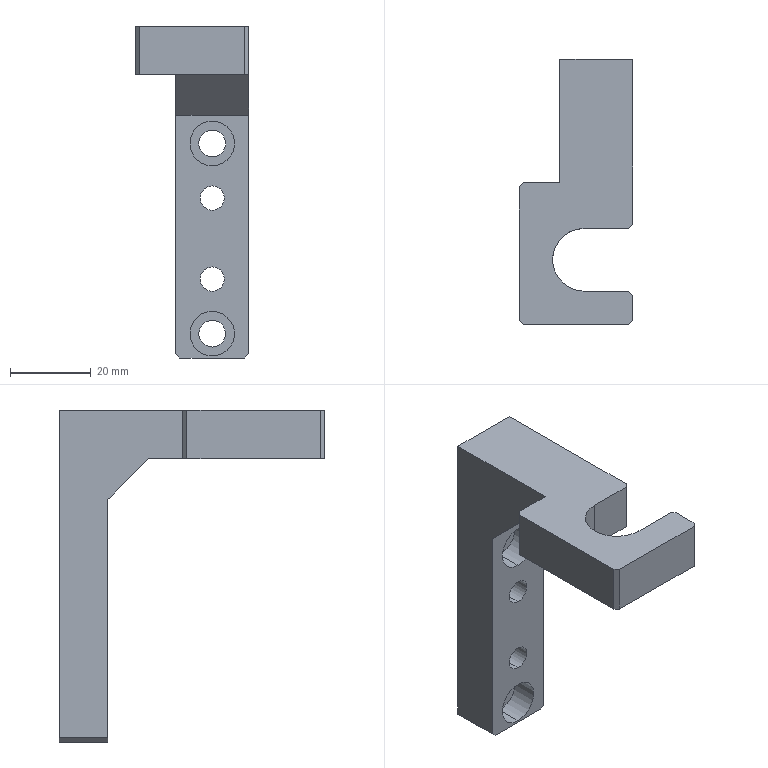Part | SolidWorks | features Chamfer 2, HoleWzd 2, ICE 2, Cut 1, Extrusion 1 | 1 solid | 36 faces | box 28 x 65.5 x 82 mm | volume 28684 mm3 | plane 23 | cylinder 13 | commonest cylinder face diameters 6 x4 6.6 x4 11 x4 15.5 x1
STEP:
#1=CARTESIAN_POINT('',(0.,32.75,-33.5));
#2=VERTEX_POINT('',#1);
#3=CARTESIAN_POINT('',(0.,32.75,-39.5));
#4=VERTEX_POINT('',#3);
#5=CARTESIAN_POINT('',(0.,32.75,-36.5));
#6=DIRECTION('',(0.,-1.,0.));
#7=DIRECTION('',(0.,0.,-1.));
#8=AXIS2_PLACEMENT_3D('',#5,#6,#7);
#9=CIRCLE('',#8,3.);
#10=EDGE_CURVE('',#2,#4,#9,.T.);
#11=ORIENTED_EDGE('',*,*,#10,.F.);
#12=CARTESIAN_POINT('',(0.,20.75,-33.5));
#13=VERTEX_POINT('',#12);
#14=CARTESIAN_POINT('',(0.,20.75,-33.5));
#15=DIRECTION('',(0.,-1.,0.));
#16=VECTOR('',#15,1000.);
#17=LINE('',#14,#16);
#18=EDGE_CURVE('',#2,#13,#17,.T.);
#19=ORIENTED_EDGE('',*,*,#18,.T.);
#20=CARTESIAN_POINT('',(0.,20.75,-39.5));
#21=VERTEX_POINT('',#20);
#22=CARTESIAN_POINT('',(0.,20.75,-36.5));
#23=DIRECTION('',(0.,-1.,0.));
#24=DIRECTION('',(0.,0.,-1.));
#25=AXIS2_PLACEMENT_3D('',#22,#23,#24);
#26=CIRCLE('',#25,3.);
#27=EDGE_CURVE('',#13,#21,#26,.T.);
#28=ORIENTED_EDGE('',*,*,#27,.T.);
#29=CARTESIAN_POINT('',(0.,20.75,-39.5));
#30=DIRECTION('',(0.,-1.,0.));
#31=VECTOR('',#30,1000.);
#32=LINE('',#29,#31);
#33=EDGE_CURVE('',#4,#21,#32,.T.);
#34=ORIENTED_EDGE('',*,*,#33,.F.);
#35=EDGE_LOOP('',(#11,#19,#28,#34));
#36=FACE_OUTER_BOUND('',#35,.T.);
#37=CARTESIAN_POINT('',(0.,20.75,-36.5));
#38=DIRECTION('',(0.,-1.,0.));
#39=DIRECTION('',(0.,0.,-1.));
#40=AXIS2_PLACEMENT_3D('',#37,#38,#39);
#41=CYLINDRICAL_SURFACE('',#40,3.);
#42=ADVANCED_FACE('',(#36),#41,.F.);
#43=CARTESIAN_POINT('',(0.,32.75,-53.5));
#44=VERTEX_POINT('',#43);
#45=CARTESIAN_POINT('',(0.,32.75,-59.5));
#46=VERTEX_POINT('',#45);
#47=CARTESIAN_POINT('',(0.,32.75,-56.5));
#48=DIRECTION('',(0.,-1.,0.));
#49=DIRECTION('',(0.,0.,-1.));
#50=AXIS2_PLACEMENT_3D('',#47,#48,#49);
#51=CIRCLE('',#50,3.);
#52=EDGE_CURVE('',#44,#46,#51,.T.);
#53=ORIENTED_EDGE('',*,*,#52,.F.);
#54=CARTESIAN_POINT('',(0.,20.75,-53.5));
#55=VERTEX_POINT('',#54);
#56=CARTESIAN_POINT('',(0.,20.75,-53.5));
#57=DIRECTION('',(0.,-1.,0.));
#58=VECTOR('',#57,1000.);
#59=LINE('',#56,#58);
#60=EDGE_CURVE('',#44,#55,#59,.T.);
#61=ORIENTED_EDGE('',*,*,#60,.T.);
#62=CARTESIAN_POINT('',(0.,20.75,-59.5));
#63=VERTEX_POINT('',#62);
#64=CARTESIAN_POINT('',(0.,20.75,-56.5));
#65=DIRECTION('',(0.,-1.,0.));
#66=DIRECTION('',(0.,0.,-1.));
#67=AXIS2_PLACEMENT_3D('',#64,#65,#66);
#68=CIRCLE('',#67,3.);
#69=EDGE_CURVE('',#55,#63,#68,.T.);
#70=ORIENTED_EDGE('',*,*,#69,.T.);
#71=CARTESIAN_POINT('',(0.,20.75,-59.5));
#72=DIRECTION('',(0.,-1.,0.));
#73=VECTOR('',#72,1000.);
#74=LINE('',#71,#73);
#75=EDGE_CURVE('',#46,#63,#74,.T.);
#76=ORIENTED_EDGE('',*,*,#75,.F.);
#77=EDGE_LOOP('',(#53,#61,#70,#76));
#78=FACE_OUTER_BOUND('',#77,.T.);
#79=CARTESIAN_POINT('',(0.,20.75,-56.5));
#80=DIRECTION('',(0.,-1.,0.));
#81=DIRECTION('',(0.,0.,-1.));
#82=AXIS2_PLACEMENT_3D('',#79,#80,#81);
#83=CYLINDRICAL_SURFACE('',#82,3.);
#84=ADVANCED_FACE('',(#78),#83,.F.);
#85=CARTESIAN_POINT('',(0.,27.15,-17.5));
#86=VERTEX_POINT('',#85);
#87=CARTESIAN_POINT('',(0.,27.15,-28.5));
#88=VERTEX_POINT('',#87);
#89=CARTESIAN_POINT('',(0.,27.15,-23.));
#90=DIRECTION('',(0.,-1.,0.));
#91=DIRECTION('',(0.,0.,-1.));
#92=AXIS2_PLACEMENT_3D('',#89,#90,#91);
#93=CIRCLE('',#92,5.5);
#94=EDGE_CURVE('',#86,#88,#93,.T.);
#95=ORIENTED_EDGE('',*,*,#94,.F.);
#96=CARTESIAN_POINT('',(0.,20.75,-17.5));
#97=VERTEX_POINT('',#96);
#98=CARTESIAN_POINT('',(0.,20.75,-17.5));
#99=DIRECTION('',(0.,-1.,0.));
#100=VECTOR('',#99,1000.);
#101=LINE('',#98,#100);
#102=EDGE_CURVE('',#86,#97,#101,.T.);
#103=ORIENTED_EDGE('',*,*,#102,.T.);
#104=CARTESIAN_POINT('',(0.,20.75,-28.5));
#105=VERTEX_POINT('',#104);
#106=CARTESIAN_POINT('',(0.,20.75,-23.));
#107=DIRECTION('',(0.,-1.,0.));
#108=DIRECTION('',(0.,0.,-1.));
#109=AXIS2_PLACEMENT_3D('',#106,#107,#108);
#110=CIRCLE('',#109,5.5);
#111=EDGE_CURVE('',#97,#105,#110,.T.);
#112=ORIENTED_EDGE('',*,*,#111,.T.);
#113=CARTESIAN_POINT('',(0.,20.75,-28.5));
#114=DIRECTION('',(0.,-1.,0.));
#115=VECTOR('',#114,1000.);
#116=LINE('',#113,#115);
#117=EDGE_CURVE('',#88,#105,#116,.T.);
#118=ORIENTED_EDGE('',*,*,#117,.F.);
#119=EDGE_LOOP('',(#95,#103,#112,#118));
#120=FACE_OUTER_BOUND('',#119,.T.);
#121=CARTESIAN_POINT('',(0.,20.75,-23.));
#122=DIRECTION('',(0.,-1.,0.));
#123=DIRECTION('',(0.,0.,-1.));
#124=AXIS2_PLACEMENT_3D('',#121,#122,#123);
#125=CYLINDRICAL_SURFACE('',#124,5.5);
#126=ADVANCED_FACE('',(#120),#125,.F.);
#127=CARTESIAN_POINT('',(0.,32.75,-19.7));
#128=VERTEX_POINT('',#127);
#129=CARTESIAN_POINT('',(0.,32.75,-26.3));
#130=VERTEX_POINT('',#129);
#131=CARTESIAN_POINT('',(0.,32.75,-23.));
#132=DIRECTION('',(0.,-1.,0.));
#133=DIRECTION('',(0.,0.,-1.));
#134=AXIS2_PLACEMENT_3D('',#131,#132,#133);
#135=CIRCLE('',#134,3.3);
#136=EDGE_CURVE('',#128,#130,#135,.T.);
#137=ORIENTED_EDGE('',*,*,#136,.F.);
#138=CARTESIAN_POINT('',(0.,27.15,-19.7));
#139=VERTEX_POINT('',#138);
#140=CARTESIAN_POINT('',(0.,20.75,-19.7));
#141=DIRECTION('',(0.,-1.,0.));
#142=VECTOR('',#141,1000.);
#143=LINE('',#140,#142);
#144=EDGE_CURVE('',#128,#139,#143,.T.);
#145=ORIENTED_EDGE('',*,*,#144,.T.);
#146=CARTESIAN_POINT('',(0.,27.15,-26.3));
#147=VERTEX_POINT('',#146);
#148=CARTESIAN_POINT('',(0.,27.15,-23.));
#149=DIRECTION('',(0.,-1.,0.));
#150=DIRECTION('',(0.,0.,-1.));
#151=AXIS2_PLACEMENT_3D('',#148,#149,#150);
#152=CIRCLE('',#151,3.3);
#153=EDGE_CURVE('',#139,#147,#152,.T.);
#154=ORIENTED_EDGE('',*,*,#153,.T.);
#155=CARTESIAN_POINT('',(0.,20.75,-26.3));
#156=DIRECTION('',(0.,-1.,0.));
#157=VECTOR('',#156,1000.);
#158=LINE('',#155,#157);
#159=EDGE_CURVE('',#130,#147,#158,.T.);
#160=ORIENTED_EDGE('',*,*,#159,.F.);
#161=EDGE_LOOP('',(#137,#145,#154,#160));
#162=FACE_OUTER_BOUND('',#161,.T.);
#163=CARTESIAN_POINT('',(0.,20.75,-23.));
#164=DIRECTION('',(0.,-1.,0.));
#165=DIRECTION('',(0.,0.,-1.));
#166=AXIS2_PLACEMENT_3D('',#163,#164,#165);
#167=CYLINDRICAL_SURFACE('',#166,3.3);
#168=ADVANCED_FACE('',(#162),#167,.F.);
#169=CARTESIAN_POINT('',(0.,27.15,-64.5));
#170=VERTEX_POINT('',#169);
#171=CARTESIAN_POINT('',(0.,27.15,-75.5));
#172=VERTEX_POINT('',#171);
#173=CARTESIAN_POINT('',(0.,27.15,-70.));
#174=DIRECTION('',(0.,-1.,0.));
#175=DIRECTION('',(0.,0.,-1.));
#176=AXIS2_PLACEMENT_3D('',#173,#174,#175);
#177=CIRCLE('',#176,5.5);
#178=EDGE_CURVE('',#170,#172,#177,.T.);
#179=ORIENTED_EDGE('',*,*,#178,.F.);
#180=CARTESIAN_POINT('',(0.,20.75,-64.5));
#181=VERTEX_POINT('',#180);
#182=CARTESIAN_POINT('',(0.,20.75,-64.5));
#183=DIRECTION('',(0.,-1.,0.));
#184=VECTOR('',#183,1000.);
#185=LINE('',#182,#184);
#186=EDGE_CURVE('',#170,#181,#185,.T.);
#187=ORIENTED_EDGE('',*,*,#186,.T.);
#188=CARTESIAN_POINT('',(0.,20.75,-75.5));
#189=VERTEX_POINT('',#188);
#190=CARTESIAN_POINT('',(0.,20.75,-70.));
#191=DIRECTION('',(0.,-1.,0.));
#192=DIRECTION('',(0.,0.,-1.));
#193=AXIS2_PLACEMENT_3D('',#190,#191,#192);
#194=CIRCLE('',#193,5.5);
#195=EDGE_CURVE('',#181,#189,#194,.T.);
#196=ORIENTED_EDGE('',*,*,#195,.T.);
#197=CARTESIAN_POINT('',(0.,20.75,-75.5));
#198=DIRECTION('',(0.,-1.,0.));
#199=VECTOR('',#198,1000.);
#200=LINE('',#197,#199);
#201=EDGE_CURVE('',#172,#189,#200,.T.);
#202=ORIENTED_EDGE('',*,*,#201,.F.);
#203=EDGE_LOOP('',(#179,#187,#196,#202));
#204=FACE_OUTER_BOUND('',#203,.T.);
#205=CARTESIAN_POINT('',(0.,20.75,-70.));
#206=DIRECTION('',(0.,-1.,0.));
#207=DIRECTION('',(0.,0.,-1.));
#208=AXIS2_PLACEMENT_3D('',#205,#206,#207);
#209=CYLINDRICAL_SURFACE('',#208,5.5);
#210=ADVANCED_FACE('',(#204),#209,.F.);
#211=CARTESIAN_POINT('',(0.,32.75,-66.7));
#212=VERTEX_POINT('',#211);
#213=CARTESIAN_POINT('',(0.,32.75,-73.3));
#214=VERTEX_POINT('',#213);
#215=CARTESIAN_POINT('',(0.,32.75,-70.));
#216=DIRECTION('',(0.,-1.,0.));
#217=DIRECTION('',(0.,0.,-1.));
#218=AXIS2_PLACEMENT_3D('',#215,#216,#217);
#219=CIRCLE('',#218,3.3);
#220=EDGE_CURVE('',#212,#214,#219,.T.);
#221=ORIENTED_EDGE('',*,*,#220,.F.);
#222=CARTESIAN_POINT('',(0.,27.15,-66.7));
#223=VERTEX_POINT('',#222);
#224=CARTESIAN_POINT('',(0.,20.75,-66.7));
#225=DIRECTION('',(0.,-1.,0.));
#226=VECTOR('',#225,1000.);
#227=LINE('',#224,#226);
#228=EDGE_CURVE('',#212,#223,#227,.T.);
#229=ORIENTED_EDGE('',*,*,#228,.T.);
#230=CARTESIAN_POINT('',(0.,27.15,-73.3));
#231=VERTEX_POINT('',#230);
#232=CARTESIAN_POINT('',(0.,27.15,-70.));
#233=DIRECTION('',(0.,-1.,0.));
#234=DIRECTION('',(0.,0.,-1.));
#235=AXIS2_PLACEMENT_3D('',#232,#233,#234);
#236=CIRCLE('',#235,3.3);
#237=EDGE_CURVE('',#223,#231,#236,.T.);
#238=ORIENTED_EDGE('',*,*,#237,.T.);
#239=CARTESIAN_POINT('',(0.,20.75,-73.3));
#240=DIRECTION('',(0.,-1.,0.));
#241=VECTOR('',#240,1000.);
#242=LINE('',#239,#241);
#243=EDGE_CURVE('',#214,#231,#242,.T.);
#244=ORIENTED_EDGE('',*,*,#243,.F.);
#245=EDGE_LOOP('',(#221,#229,#238,#244));
#246=FACE_OUTER_BOUND('',#245,.T.);
#247=CARTESIAN_POINT('',(0.,20.75,-70.));
#248=DIRECTION('',(0.,-1.,0.));
#249=DIRECTION('',(0.,0.,-1.));
#250=AXIS2_PLACEMENT_3D('',#247,#248,#249);
#251=CYLINDRICAL_SURFACE('',#250,3.3);
#252=ADVANCED_FACE('',(#246),#251,.F.);
#253=CARTESIAN_POINT('',(9.,-8.,6.));
#254=VERTEX_POINT('',#253);
#255=CARTESIAN_POINT('',(9.,32.75,6.));
#256=VERTEX_POINT('',#255);
#257=CARTESIAN_POINT('',(9.,-32.75,6.));
#258=DIRECTION('',(0.,1.,0.));
#259=VECTOR('',#258,1000.);
#260=LINE('',#257,#259);
#261=EDGE_CURVE('',#254,#256,#260,.T.);
#262=ORIENTED_EDGE('',*,*,#261,.F.);
#263=CARTESIAN_POINT('',(9.,-8.,-6.));
#264=VERTEX_POINT('',#263);
#265=CARTESIAN_POINT('',(9.,-8.,6.));
#266=DIRECTION('',(0.,0.,-1.));
#267=VECTOR('',#266,1000.);
#268=LINE('',#265,#267);
#269=EDGE_CURVE('',#254,#264,#268,.T.);
#270=ORIENTED_EDGE('',*,*,#269,.T.);
#271=CARTESIAN_POINT('',(9.,10.75,-6.));
#272=VERTEX_POINT('',#271);
#273=CARTESIAN_POINT('',(9.,-32.75,-6.));
#274=DIRECTION('',(0.,1.,0.));
#275=VECTOR('',#274,1000.);
#276=LINE('',#273,#275);
#277=EDGE_CURVE('',#264,#272,#276,.T.);
#278=ORIENTED_EDGE('',*,*,#277,.T.);
#279=CARTESIAN_POINT('',(9.,20.75,-16.));
#280=VERTEX_POINT('',#279);
#281=CARTESIAN_POINT('',(9.,-17.,21.75));
#282=DIRECTION('',(0.,0.7071,-0.7071));
#283=VECTOR('',#282,1000.);
#284=LINE('',#281,#283);
#285=EDGE_CURVE('',#272,#280,#284,.T.);
#286=ORIENTED_EDGE('',*,*,#285,.T.);
#287=CARTESIAN_POINT('',(9.,20.75,-75.));
#288=VERTEX_POINT('',#287);
#289=CARTESIAN_POINT('',(9.,20.75,-76.));
#290=DIRECTION('',(0.,0.,1.));
#291=VECTOR('',#290,1000.);
#292=LINE('',#289,#291);
#293=EDGE_CURVE('',#288,#280,#292,.T.);
#294=ORIENTED_EDGE('',*,*,#293,.F.);
#295=CARTESIAN_POINT('',(9.,32.75,-75.));
#296=VERTEX_POINT('',#295);
#297=CARTESIAN_POINT('',(9.,-32.75,-75.));
#298=DIRECTION('',(0.,1.,0.));
#299=VECTOR('',#298,1000.);
#300=LINE('',#297,#299);
#301=EDGE_CURVE('',#288,#296,#300,.T.);
#302=ORIENTED_EDGE('',*,*,#301,.T.);
#303=CARTESIAN_POINT('',(9.,32.75,6.));
#304=DIRECTION('',(0.,0.,-1.));
#305=VECTOR('',#304,1000.);
#306=LINE('',#303,#305);
#307=EDGE_CURVE('',#256,#296,#306,.T.);
#308=ORIENTED_EDGE('',*,*,#307,.F.);
#309=EDGE_LOOP('',(#262,#270,#278,#286,#294,#302,#308));
#310=FACE_OUTER_BOUND('',#309,.T.);
#311=CARTESIAN_POINT('',(9.,-32.75,6.));
#312=DIRECTION('',(-1.,0.,0.));
#313=DIRECTION('',(0.,0.,1.));
#314=AXIS2_PLACEMENT_3D('',#311,#312,#313);
#315=PLANE('',#314);
#316=ADVANCED_FACE('',(#310),#315,.F.);
#317=CARTESIAN_POINT('',(9.,-31.75,-6.));
#318=VERTEX_POINT('',#317);
#319=CARTESIAN_POINT('',(9.,-25.5,-6.));
#320=VERTEX_POINT('',#319);
#321=CARTESIAN_POINT('',(9.,-32.75,-6.));
#322=DIRECTION('',(0.,1.,0.));
#323=VECTOR('',#322,1000.);
#324=LINE('',#321,#323);
#325=EDGE_CURVE('',#318,#320,#324,.T.);
#326=ORIENTED_EDGE('',*,*,#325,.T.);
#327=CARTESIAN_POINT('',(9.,-25.5,6.));
#328=VERTEX_POINT('',#327);
#329=CARTESIAN_POINT('',(9.,-25.5,6.));
#330=DIRECTION('',(0.,0.,1.));
#331=VECTOR('',#330,1000.);
#332=LINE('',#329,#331);
#333=EDGE_CURVE('',#320,#328,#332,.T.);
#334=ORIENTED_EDGE('',*,*,#333,.T.);
#335=CARTESIAN_POINT('',(9.,-31.75,6.));
#336=VERTEX_POINT('',#335);
#337=CARTESIAN_POINT('',(9.,-32.75,6.));
#338=DIRECTION('',(0.,1.,0.));
#339=VECTOR('',#338,1000.);
#340=LINE('',#337,#339);
#341=EDGE_CURVE('',#336,#328,#340,.T.);
#342=ORIENTED_EDGE('',*,*,#341,.F.);
#343=CARTESIAN_POINT('',(9.,-31.75,6.));
#344=DIRECTION('',(0.,0.,-1.));
#345=VECTOR('',#344,1000.);
#346=LINE('',#343,#345);
#347=EDGE_CURVE('',#336,#318,#346,.T.);
#348=ORIENTED_EDGE('',*,*,#347,.T.);
#349=EDGE_LOOP('',(#326,#334,#342,#348));
#350=FACE_OUTER_BOUND('',#349,.T.);
#351=CARTESIAN_POINT('',(9.,-32.75,6.));
#352=DIRECTION('',(-1.,0.,0.));
#353=DIRECTION('',(0.,0.,1.));
#354=AXIS2_PLACEMENT_3D('',#351,#352,#353);
#355=PLANE('',#354);
#356=ADVANCED_FACE('',(#350),#355,.F.);
#357=CARTESIAN_POINT('',(0.,32.75,-36.5));
#358=DIRECTION('',(0.,-1.,0.));
#359=DIRECTION('',(0.,0.,-1.));
#360=AXIS2_PLACEMENT_3D('',#357,#358,#359);
#361=CIRCLE('',#360,3.);
#362=EDGE_CURVE('',#4,#2,#361,.T.);
#363=ORIENTED_EDGE('',*,*,#362,.T.);
#364=ORIENTED_EDGE('',*,*,#10,.T.);
#365=EDGE_LOOP('',(#363,#364));
#366=FACE_BOUND('',#365,.T.);
#367=CARTESIAN_POINT('',(0.,32.75,-56.5));
#368=DIRECTION('',(0.,-1.,0.));
#369=DIRECTION('',(0.,0.,-1.));
#370=AXIS2_PLACEMENT_3D('',#367,#368,#369);
#371=CIRCLE('',#370,3.);
#372=EDGE_CURVE('',#46,#44,#371,.T.);
#373=ORIENTED_EDGE('',*,*,#372,.T.);
#374=ORIENTED_EDGE('',*,*,#52,.T.);
#375=EDGE_LOOP('',(#373,#374));
#376=FACE_BOUND('',#375,.T.);
#377=CARTESIAN_POINT('',(0.,32.75,-23.));
#378=DIRECTION('',(0.,-1.,0.));
#379=DIRECTION('',(0.,0.,-1.));
#380=AXIS2_PLACEMENT_3D('',#377,#378,#379);
#381=CIRCLE('',#380,3.3);
#382=EDGE_CURVE('',#130,#128,#381,.T.);
#383=ORIENTED_EDGE('',*,*,#382,.T.);
#384=ORIENTED_EDGE('',*,*,#136,.T.);
#385=EDGE_LOOP('',(#383,#384));
#386=FACE_BOUND('',#385,.T.);
#387=CARTESIAN_POINT('',(0.,32.75,-70.));
#388=DIRECTION('',(0.,-1.,0.));
#389=DIRECTION('',(0.,0.,-1.));
#390=AXIS2_PLACEMENT_3D('',#387,#388,#389);
#391=CIRCLE('',#390,3.3);
#392=EDGE_CURVE('',#214,#212,#391,.T.);
#393=ORIENTED_EDGE('',*,*,#392,.T.);
#394=ORIENTED_EDGE('',*,*,#220,.T.);
#395=EDGE_LOOP('',(#393,#394));
#396=FACE_BOUND('',#395,.T.);
#397=CARTESIAN_POINT('',(-8.,32.75,-76.));
#398=VERTEX_POINT('',#397);
#399=CARTESIAN_POINT('',(8.,32.75,-76.));
#400=VERTEX_POINT('',#399);
#401=CARTESIAN_POINT('',(-9.,32.75,-76.));
#402=DIRECTION('',(1.,0.,0.));
#403=VECTOR('',#402,1000.);
#404=LINE('',#401,#403);
#405=EDGE_CURVE('',#398,#400,#404,.T.);
#406=ORIENTED_EDGE('',*,*,#405,.F.);
#407=CARTESIAN_POINT('',(-9.,32.75,-75.));
#408=VERTEX_POINT('',#407);
#409=CARTESIAN_POINT('',(-8.,32.75,-76.));
#410=DIRECTION('',(-0.7071,0.,0.7071));
#411=VECTOR('',#410,1000.);
#412=LINE('',#409,#411);
#413=EDGE_CURVE('',#398,#408,#412,.T.);
#414=ORIENTED_EDGE('',*,*,#413,.T.);
#415=CARTESIAN_POINT('',(-9.,32.75,6.));
#416=VERTEX_POINT('',#415);
#417=CARTESIAN_POINT('',(-9.,32.75,6.));
#418=DIRECTION('',(0.,0.,-1.));
#419=VECTOR('',#418,1000.);
#420=LINE('',#417,#419);
#421=EDGE_CURVE('',#416,#408,#420,.T.);
#422=ORIENTED_EDGE('',*,*,#421,.F.);
#423=CARTESIAN_POINT('',(-9.,32.75,6.));
#424=DIRECTION('',(-1.,0.,0.));
#425=VECTOR('',#424,1000.);
#426=LINE('',#423,#425);
#427=EDGE_CURVE('',#256,#416,#426,.T.);
#428=ORIENTED_EDGE('',*,*,#427,.F.);
#429=ORIENTED_EDGE('',*,*,#307,.T.);
#430=CARTESIAN_POINT('',(8.,32.75,-76.));
#431=DIRECTION('',(-0.7071,0.,-0.7071));
#432=VECTOR('',#431,1000.);
#433=LINE('',#430,#432);
#434=EDGE_CURVE('',#296,#400,#433,.T.);
#435=ORIENTED_EDGE('',*,*,#434,.T.);
#436=EDGE_LOOP('',(#406,#414,#422,#428,#429,#435));
#437=FACE_OUTER_BOUND('',#436,.T.);
#438=CARTESIAN_POINT('',(-9.,32.75,6.));
#439=DIRECTION('',(0.,-1.,0.));
#440=DIRECTION('',(0.,0.,-1.));
#441=AXIS2_PLACEMENT_3D('',#438,#439,#440);
#442=PLANE('',#441);
#443=ADVANCED_FACE('',(#366,#376,#386,#396,#437),#442,.F.);
#444=ORIENTED_EDGE('',*,*,#421,.T.);
#445=CARTESIAN_POINT('',(-9.,20.75,-75.));
#446=VERTEX_POINT('',#445);
#447=CARTESIAN_POINT('',(-9.,-32.75,-75.));
#448=DIRECTION('',(0.,-1.,0.));
#449=VECTOR('',#448,1000.);
#450=LINE('',#447,#449);
#451=EDGE_CURVE('',#408,#446,#450,.T.);
#452=ORIENTED_EDGE('',*,*,#451,.T.);
#453=CARTESIAN_POINT('',(-9.,20.75,-16.));
#454=VERTEX_POINT('',#453);
#455=CARTESIAN_POINT('',(-9.,20.75,-76.));
#456=DIRECTION('',(0.,0.,1.));
#457=VECTOR('',#456,1000.);
#458=LINE('',#455,#457);
#459=EDGE_CURVE('',#446,#454,#458,.T.);
#460=ORIENTED_EDGE('',*,*,#459,.T.);
#461=CARTESIAN_POINT('',(-9.,10.75,-6.));
#462=VERTEX_POINT('',#461);
#463=CARTESIAN_POINT('',(-9.,-17.,21.75));
#464=DIRECTION('',(0.,-0.7071,0.7071));
#465=VECTOR('',#464,1000.);
#466=LINE('',#463,#465);
#467=EDGE_CURVE('',#454,#462,#466,.T.);
#468=ORIENTED_EDGE('',*,*,#467,.T.);
#469=CARTESIAN_POINT('',(-9.,2.25,-6.));
#470=VERTEX_POINT('',#469);
#471=CARTESIAN_POINT('',(-9.,-32.75,-6.));
#472=DIRECTION('',(0.,-1.,0.));
#473=VECTOR('',#472,1000.);
#474=LINE('',#471,#473);
#475=EDGE_CURVE('',#462,#470,#474,.T.);
#476=ORIENTED_EDGE('',*,*,#475,.T.);
#477=CARTESIAN_POINT('',(-9.,2.25,6.));
#478=VERTEX_POINT('',#477);
#479=CARTESIAN_POINT('',(-9.,2.25,6.));
#480=DIRECTION('',(0.,0.,1.));
#481=VECTOR('',#480,1000.);
#482=LINE('',#479,#481);
#483=EDGE_CURVE('',#470,#478,#482,.T.);
#484=ORIENTED_EDGE('',*,*,#483,.T.);
#485=CARTESIAN_POINT('',(-9.,-32.75,6.));
#486=DIRECTION('',(0.,-1.,0.));
#487=VECTOR('',#486,1000.);
#488=LINE('',#485,#487);
#489=EDGE_CURVE('',#416,#478,#488,.T.);
#490=ORIENTED_EDGE('',*,*,#489,.F.);
#491=EDGE_LOOP('',(#444,#452,#460,#468,#476,#484,#490));
#492=FACE_OUTER_BOUND('',#491,.T.);
#493=CARTESIAN_POINT('',(-9.,-32.75,6.));
#494=DIRECTION('',(1.,0.,0.));
#495=DIRECTION('',(0.,0.,-1.));
#496=AXIS2_PLACEMENT_3D('',#493,#494,#495);
#497=PLANE('',#496);
#498=ADVANCED_FACE('',(#492),#497,.F.);
#499=CARTESIAN_POINT('',(-18.,-32.75,6.));
#500=VERTEX_POINT('',#499);
#501=CARTESIAN_POINT('',(8.,-32.75,6.));
#502=VERTEX_POINT('',#501);
#503=CARTESIAN_POINT('',(-9.,-32.75,6.));
#504=DIRECTION('',(1.,0.,0.));
#505=VECTOR('',#504,1000.);
#506=LINE('',#503,#505);
#507=EDGE_CURVE('',#500,#502,#506,.T.);
#508=ORIENTED_EDGE('',*,*,#507,.F.);
#509=CARTESIAN_POINT('',(-18.,-32.75,-6.));
#510=VERTEX_POINT('',#509);
#511=CARTESIAN_POINT('',(-18.,-32.75,-6.));
#512=DIRECTION('',(0.,0.,-1.));
#513=VECTOR('',#512,1000.);
#514=LINE('',#511,#513);
#515=EDGE_CURVE('',#500,#510,#514,.T.);
#516=ORIENTED_EDGE('',*,*,#515,.T.);
#517=CARTESIAN_POINT('',(8.,-32.75,-6.));
#518=VERTEX_POINT('',#517);
#519=CARTESIAN_POINT('',(-9.,-32.75,-6.));
#520=DIRECTION('',(1.,0.,0.));
#521=VECTOR('',#520,1000.);
#522=LINE('',#519,#521);
#523=EDGE_CURVE('',#510,#518,#522,.T.);
#524=ORIENTED_EDGE('',*,*,#523,.T.);
#525=CARTESIAN_POINT('',(8.,-32.75,6.));
#526=DIRECTION('',(0.,0.,1.));
#527=VECTOR('',#526,1000.);
#528=LINE('',#525,#527);
#529=EDGE_CURVE('',#518,#502,#528,.T.);
#530=ORIENTED_EDGE('',*,*,#529,.T.);
#531=EDGE_LOOP('',(#508,#516,#524,#530));
#532=FACE_OUTER_BOUND('',#531,.T.);
#533=CARTESIAN_POINT('',(-9.,-32.75,6.));
#534=DIRECTION('',(0.,1.,0.));
#535=DIRECTION('',(0.,0.,1.));
#536=AXIS2_PLACEMENT_3D('',#533,#534,#535);
#537=PLANE('',#536);
#538=ADVANCED_FACE('',(#532),#537,.F.);
#539=ORIENTED_EDGE('',*,*,#341,.T.);
#540=CARTESIAN_POINT('',(8.,-24.5,6.));
#541=VERTEX_POINT('',#540);
#542=CARTESIAN_POINT('',(9.,-25.5,6.));
#543=DIRECTION('',(-0.7071,0.7071,0.));
#544=VECTOR('',#543,1000.);
#545=LINE('',#542,#544);
#546=EDGE_CURVE('',#328,#541,#545,.T.);
#547=ORIENTED_EDGE('',*,*,#546,.T.);
#548=CARTESIAN_POINT('',(-3.,-24.5,6.));
#549=VERTEX_POINT('',#548);
#550=CARTESIAN_POINT('',(-3.,-24.5,6.));
#551=DIRECTION('',(1.,0.,0.));
#552=VECTOR('',#551,1000.);
#553=LINE('',#550,#552);
#554=EDGE_CURVE('',#549,#541,#553,.T.);
#555=ORIENTED_EDGE('',*,*,#554,.F.);
#556=CARTESIAN_POINT('',(-3.,-9.,6.));
#557=VERTEX_POINT('',#556);
#558=CARTESIAN_POINT('',(-3.,-16.75,6.));
#559=DIRECTION('',(0.,0.,1.));
#560=DIRECTION('',(1.,0.,0.));
#561=AXIS2_PLACEMENT_3D('',#558,#559,#560);
#562=CIRCLE('',#561,7.75);
#563=EDGE_CURVE('',#557,#549,#562,.T.);
#564=ORIENTED_EDGE('',*,*,#563,.F.);
#565=CARTESIAN_POINT('',(8.,-9.,6.));
#566=VERTEX_POINT('',#565);
#567=CARTESIAN_POINT('',(-3.,-9.,6.));
#568=DIRECTION('',(-1.,0.,0.));
#569=VECTOR('',#568,1000.);
#570=LINE('',#567,#569);
#571=EDGE_CURVE('',#566,#557,#570,.T.);
#572=ORIENTED_EDGE('',*,*,#571,.F.);
#573=CARTESIAN_POINT('',(9.,-8.,6.));
#574=DIRECTION('',(0.7071,0.7071,0.));
#575=VECTOR('',#574,1000.);
#576=LINE('',#573,#575);
#577=EDGE_CURVE('',#566,#254,#576,.T.);
#578=ORIENTED_EDGE('',*,*,#577,.T.);
#579=ORIENTED_EDGE('',*,*,#261,.T.);
#580=ORIENTED_EDGE('',*,*,#427,.T.);
#581=ORIENTED_EDGE('',*,*,#489,.T.);
#582=CARTESIAN_POINT('',(-18.,2.25,6.));
#583=VERTEX_POINT('',#582);
#584=CARTESIAN_POINT('',(-19.,2.25,6.));
#585=DIRECTION('',(-1.,0.,0.));
#586=VECTOR('',#585,1000.);
#587=LINE('',#584,#586);
#588=EDGE_CURVE('',#478,#583,#587,.T.);
#589=ORIENTED_EDGE('',*,*,#588,.T.);
#590=CARTESIAN_POINT('',(-19.,1.25,6.));
#591=VERTEX_POINT('',#590);
#592=CARTESIAN_POINT('',(-18.,2.25,6.));
#593=DIRECTION('',(-0.7071,-0.7071,0.));
#594=VECTOR('',#593,1000.);
#595=LINE('',#592,#594);
#596=EDGE_CURVE('',#583,#591,#595,.T.);
#597=ORIENTED_EDGE('',*,*,#596,.T.);
#598=CARTESIAN_POINT('',(-19.,-31.75,6.));
#599=VERTEX_POINT('',#598);
#600=CARTESIAN_POINT('',(-19.,2.25,6.));
#601=DIRECTION('',(0.,-1.,0.));
#602=VECTOR('',#601,1000.);
#603=LINE('',#600,#602);
#604=EDGE_CURVE('',#591,#599,#603,.T.);
#605=ORIENTED_EDGE('',*,*,#604,.T.);
#606=CARTESIAN_POINT('',(-19.,-31.75,6.));
#607=DIRECTION('',(0.7071,-0.7071,0.));
#608=VECTOR('',#607,1000.);
#609=LINE('',#606,#608);
#610=EDGE_CURVE('',#599,#500,#609,.T.);
#611=ORIENTED_EDGE('',*,*,#610,.T.);
#612=ORIENTED_EDGE('',*,*,#507,.T.);
#613=CARTESIAN_POINT('',(9.,-31.75,6.));
#614=DIRECTION('',(0.7071,0.7071,0.));
#615=VECTOR('',#614,1000.);
#616=LINE('',#613,#615);
#617=EDGE_CURVE('',#502,#336,#616,.T.);
#618=ORIENTED_EDGE('',*,*,#617,.T.);
#619=EDGE_LOOP('',(#539,#547,#555,#564,#572,#578,#579,#580,#581,#589,#597,#605,#611,#612,#618));
#620=FACE_OUTER_BOUND('',#619,.T.);
#621=CARTESIAN_POINT('',(0.,0.,6.));
#622=DIRECTION('',(0.,0.,-1.));
#623=DIRECTION('',(-1.,0.,0.));
#624=AXIS2_PLACEMENT_3D('',#621,#622,#623);
#625=PLANE('',#624);
#626=ADVANCED_FACE('',(#620),#625,.F.);
#627=CARTESIAN_POINT('',(-3.,-24.5,-6.));
#628=VERTEX_POINT('',#627);
#629=CARTESIAN_POINT('',(8.,-24.5,-6.));
#630=VERTEX_POINT('',#629);
#631=CARTESIAN_POINT('',(-3.,-24.5,-6.));
#632=DIRECTION('',(1.,0.,0.));
#633=VECTOR('',#632,1000.);
#634=LINE('',#631,#633);
#635=EDGE_CURVE('',#628,#630,#634,.T.);
#636=ORIENTED_EDGE('',*,*,#635,.T.);
#637=CARTESIAN_POINT('',(-8.25,-8.25,-6.));
#638=DIRECTION('',(0.7071,-0.7071,0.));
#639=VECTOR('',#638,1000.);
#640=LINE('',#637,#639);
#641=EDGE_CURVE('',#630,#320,#640,.T.);
#642=ORIENTED_EDGE('',*,*,#641,.T.);
#643=ORIENTED_EDGE('',*,*,#325,.F.);
#644=CARTESIAN_POINT('',(20.375,-20.375,-6.));
#645=DIRECTION('',(-0.7071,-0.7071,0.));
#646=VECTOR('',#645,1000.);
#647=LINE('',#644,#646);
#648=EDGE_CURVE('',#318,#518,#647,.T.);
#649=ORIENTED_EDGE('',*,*,#648,.T.);
#650=ORIENTED_EDGE('',*,*,#523,.F.);
#651=CARTESIAN_POINT('',(-19.,-31.75,-6.));
#652=VERTEX_POINT('',#651);
#653=CARTESIAN_POINT('',(-25.375,-25.375,-6.));
#654=DIRECTION('',(-0.7071,0.7071,0.));
#655=VECTOR('',#654,1000.);
#656=LINE('',#653,#655);
#657=EDGE_CURVE('',#510,#652,#656,.T.);
#658=ORIENTED_EDGE('',*,*,#657,.T.);
#659=CARTESIAN_POINT('',(-19.,1.25,-6.));
#660=VERTEX_POINT('',#659);
#661=CARTESIAN_POINT('',(-19.,2.25,-6.));
#662=DIRECTION('',(0.,-1.,0.));
#663=VECTOR('',#662,1000.);
#664=LINE('',#661,#663);
#665=EDGE_CURVE('',#660,#652,#664,.T.);
#666=ORIENTED_EDGE('',*,*,#665,.F.);
#667=CARTESIAN_POINT('',(-18.,2.25,-6.));
#668=VERTEX_POINT('',#667);
#669=CARTESIAN_POINT('',(-10.125,10.125,-6.));
#670=DIRECTION('',(0.7071,0.7071,0.));
#671=VECTOR('',#670,1000.);
#672=LINE('',#669,#671);
#673=EDGE_CURVE('',#660,#668,#672,.T.);
#674=ORIENTED_EDGE('',*,*,#673,.T.);
#675=CARTESIAN_POINT('',(-19.,2.25,-6.));
#676=DIRECTION('',(-1.,0.,0.));
#677=VECTOR('',#676,1000.);
#678=LINE('',#675,#677);
#679=EDGE_CURVE('',#470,#668,#678,.T.);
#680=ORIENTED_EDGE('',*,*,#679,.F.);
#681=ORIENTED_EDGE('',*,*,#475,.F.);
#682=CARTESIAN_POINT('',(0.,10.75,-6.));
#683=DIRECTION('',(1.,0.,0.));
#684=VECTOR('',#683,1000.);
#685=LINE('',#682,#684);
#686=EDGE_CURVE('',#462,#272,#685,.T.);
#687=ORIENTED_EDGE('',*,*,#686,.T.);
#688=ORIENTED_EDGE('',*,*,#277,.F.);
#689=CARTESIAN_POINT('',(8.,-9.,-6.));
#690=VERTEX_POINT('',#689);
#691=CARTESIAN_POINT('',(8.5,-8.5,-6.));
#692=DIRECTION('',(-0.7071,-0.7071,0.));
#693=VECTOR('',#692,1000.);
#694=LINE('',#691,#693);
#695=EDGE_CURVE('',#264,#690,#694,.T.);
#696=ORIENTED_EDGE('',*,*,#695,.T.);
#697=CARTESIAN_POINT('',(-3.,-9.,-6.));
#698=VERTEX_POINT('',#697);
#699=CARTESIAN_POINT('',(0.,-9.,-6.));
#700=DIRECTION('',(1.,0.,0.));
#701=VECTOR('',#700,1000.);
#702=LINE('',#699,#701);
#703=EDGE_CURVE('',#698,#690,#702,.T.);
#704=ORIENTED_EDGE('',*,*,#703,.F.);
#705=CARTESIAN_POINT('',(-3.,-16.75,-6.));
#706=DIRECTION('',(0.,0.,1.));
#707=DIRECTION('',(1.,0.,0.));
#708=AXIS2_PLACEMENT_3D('',#705,#706,#707);
#709=CIRCLE('',#708,7.75);
#710=EDGE_CURVE('',#698,#628,#709,.T.);
#711=ORIENTED_EDGE('',*,*,#710,.T.);
#712=EDGE_LOOP('',(#636,#642,#643,#649,#650,#658,#666,#674,#680,#681,#687,#688,#696,#704,#711));
#713=FACE_OUTER_BOUND('',#712,.T.);
#714=CARTESIAN_POINT('',(0.,0.,-6.));
#715=DIRECTION('',(0.,0.,-1.));
#716=DIRECTION('',(-1.,0.,0.));
#717=AXIS2_PLACEMENT_3D('',#714,#715,#716);
#718=PLANE('',#717);
#719=ADVANCED_FACE('',(#713),#718,.T.);
#720=ORIENTED_EDGE('',*,*,#679,.T.);
#721=CARTESIAN_POINT('',(-18.,2.25,-50.822));
#722=DIRECTION('',(0.,0.,1.));
#723=VECTOR('',#722,1000.);
#724=LINE('',#721,#723);
#725=EDGE_CURVE('',#668,#583,#724,.T.);
#726=ORIENTED_EDGE('',*,*,#725,.T.);
#727=ORIENTED_EDGE('',*,*,#588,.F.);
#728=ORIENTED_EDGE('',*,*,#483,.F.);
#729=EDGE_LOOP('',(#720,#726,#727,#728));
#730=FACE_OUTER_BOUND('',#729,.T.);
#731=CARTESIAN_POINT('',(-19.,2.25,-50.822));
#732=DIRECTION('',(0.,1.,0.));
#733=DIRECTION('',(0.,0.,1.));
#734=AXIS2_PLACEMENT_3D('',#731,#732,#733);
#735=PLANE('',#734);
#736=ADVANCED_FACE('',(#730),#735,.T.);
#737=ORIENTED_EDGE('',*,*,#604,.F.);
#738=CARTESIAN_POINT('',(-19.,1.25,-50.822));
#739=DIRECTION('',(0.,0.,-1.));
#740=VECTOR('',#739,1000.);
#741=LINE('',#738,#740);
#742=EDGE_CURVE('',#591,#660,#741,.T.);
#743=ORIENTED_EDGE('',*,*,#742,.T.);
#744=ORIENTED_EDGE('',*,*,#665,.T.);
#745=CARTESIAN_POINT('',(-19.,-31.75,6.));
#746=DIRECTION('',(0.,0.,1.));
#747=VECTOR('',#746,1000.);
#748=LINE('',#745,#747);
#749=EDGE_CURVE('',#652,#599,#748,.T.);
#750=ORIENTED_EDGE('',*,*,#749,.T.);
#751=EDGE_LOOP('',(#737,#743,#744,#750));
#752=FACE_OUTER_BOUND('',#751,.T.);
#753=CARTESIAN_POINT('',(-19.,2.25,-50.822));
#754=DIRECTION('',(-1.,0.,0.));
#755=DIRECTION('',(0.,-1.,0.));
#756=AXIS2_PLACEMENT_3D('',#753,#754,#755);
#757=PLANE('',#756);
#758=ADVANCED_FACE('',(#752),#757,.T.);
#759=ORIENTED_EDGE('',*,*,#703,.T.);
#760=CARTESIAN_POINT('',(8.,-9.,-6.));
#761=DIRECTION('',(0.,0.,1.));
#762=VECTOR('',#761,1000.);
#763=LINE('',#760,#762);
#764=EDGE_CURVE('',#690,#566,#763,.T.);
#765=ORIENTED_EDGE('',*,*,#764,.T.);
#766=ORIENTED_EDGE('',*,*,#571,.T.);
#767=CARTESIAN_POINT('',(-3.,-9.,-6.));
#768=DIRECTION('',(0.,0.,1.));
#769=VECTOR('',#768,1000.);
#770=LINE('',#767,#769);
#771=EDGE_CURVE('',#698,#557,#770,.T.);
#772=ORIENTED_EDGE('',*,*,#771,.F.);
#773=EDGE_LOOP('',(#759,#765,#766,#772));
#774=FACE_OUTER_BOUND('',#773,.T.);
#775=CARTESIAN_POINT('',(-3.,-9.,-6.));
#776=DIRECTION('',(0.,1.,0.));
#777=DIRECTION('',(0.,0.,1.));
#778=AXIS2_PLACEMENT_3D('',#775,#776,#777);
#779=PLANE('',#778);
#780=ADVANCED_FACE('',(#774),#779,.F.);
#781=ORIENTED_EDGE('',*,*,#554,.T.);
#782=CARTESIAN_POINT('',(8.,-24.5,-6.));
#783=DIRECTION('',(0.,0.,-1.));
#784=VECTOR('',#783,1000.);
#785=LINE('',#782,#784);
#786=EDGE_CURVE('',#541,#630,#785,.T.);
#787=ORIENTED_EDGE('',*,*,#786,.T.);
#788=ORIENTED_EDGE('',*,*,#635,.F.);
#789=CARTESIAN_POINT('',(-3.,-24.5,-6.));
#790=DIRECTION('',(0.,0.,1.));
#791=VECTOR('',#790,1000.);
#792=LINE('',#789,#791);
#793=EDGE_CURVE('',#628,#549,#792,.T.);
#794=ORIENTED_EDGE('',*,*,#793,.T.);
#795=EDGE_LOOP('',(#781,#787,#788,#794));
#796=FACE_OUTER_BOUND('',#795,.T.);
#797=CARTESIAN_POINT('',(-3.,-24.5,-6.));
#798=DIRECTION('',(0.,-1.,0.));
#799=DIRECTION('',(0.,0.,-1.));
#800=AXIS2_PLACEMENT_3D('',#797,#798,#799);
#801=PLANE('',#800);
#802=ADVANCED_FACE('',(#796),#801,.F.);
#803=ORIENTED_EDGE('',*,*,#563,.T.);
#804=ORIENTED_EDGE('',*,*,#793,.F.);
#805=ORIENTED_EDGE('',*,*,#710,.F.);
#806=ORIENTED_EDGE('',*,*,#771,.T.);
#807=EDGE_LOOP('',(#803,#804,#805,#806));
#808=FACE_OUTER_BOUND('',#807,.T.);
#809=CARTESIAN_POINT('',(-3.,-16.75,-6.));
#810=DIRECTION('',(0.,0.,1.));
#811=DIRECTION('',(1.,0.,0.));
#812=AXIS2_PLACEMENT_3D('',#809,#810,#811);
#813=CYLINDRICAL_SURFACE('',#812,7.75);
#814=ADVANCED_FACE('',(#808),#813,.F.);
#815=CARTESIAN_POINT('',(0.,20.75,-36.5));
#816=DIRECTION('',(0.,-1.,0.));
#817=DIRECTION('',(0.,0.,-1.));
#818=AXIS2_PLACEMENT_3D('',#815,#816,#817);
#819=CIRCLE('',#818,3.);
#820=EDGE_CURVE('',#21,#13,#819,.T.);
#821=ORIENTED_EDGE('',*,*,#820,.F.);
#822=ORIENTED_EDGE('',*,*,#27,.F.);
#823=EDGE_LOOP('',(#821,#822));
#824=FACE_BOUND('',#823,.T.);
#825=CARTESIAN_POINT('',(0.,20.75,-56.5));
#826=DIRECTION('',(0.,-1.,0.));
#827=DIRECTION('',(0.,0.,-1.));
#828=AXIS2_PLACEMENT_3D('',#825,#826,#827);
#829=CIRCLE('',#828,3.);
#830=EDGE_CURVE('',#63,#55,#829,.T.);
#831=ORIENTED_EDGE('',*,*,#830,.F.);
#832=ORIENTED_EDGE('',*,*,#69,.F.);
#833=EDGE_LOOP('',(#831,#832));
#834=FACE_BOUND('',#833,.T.);
#835=CARTESIAN_POINT('',(0.,20.75,-23.));
#836=DIRECTION('',(0.,-1.,0.));
#837=DIRECTION('',(0.,0.,-1.));
#838=AXIS2_PLACEMENT_3D('',#835,#836,#837);
#839=CIRCLE('',#838,5.5);
#840=EDGE_CURVE('',#105,#97,#839,.T.);
#841=ORIENTED_EDGE('',*,*,#840,.F.);
#842=ORIENTED_EDGE('',*,*,#111,.F.);
#843=EDGE_LOOP('',(#841,#842));
#844=FACE_BOUND('',#843,.T.);
#845=CARTESIAN_POINT('',(0.,20.75,-70.));
#846=DIRECTION('',(0.,-1.,0.));
#847=DIRECTION('',(0.,0.,-1.));
#848=AXIS2_PLACEMENT_3D('',#845,#846,#847);
#849=CIRCLE('',#848,5.5);
#850=EDGE_CURVE('',#189,#181,#849,.T.);
#851=ORIENTED_EDGE('',*,*,#850,.F.);
#852=ORIENTED_EDGE('',*,*,#195,.F.);
#853=EDGE_LOOP('',(#851,#852));
#854=FACE_BOUND('',#853,.T.);
#855=ORIENTED_EDGE('',*,*,#459,.F.);
#856=CARTESIAN_POINT('',(-8.,20.75,-76.));
#857=VERTEX_POINT('',#856);
#858=CARTESIAN_POINT('',(-8.,20.75,-76.));
#859=DIRECTION('',(0.7071,0.,-0.7071));
#860=VECTOR('',#859,1000.);
#861=LINE('',#858,#860);
#862=EDGE_CURVE('',#446,#857,#861,.T.);
#863=ORIENTED_EDGE('',*,*,#862,.T.);
#864=CARTESIAN_POINT('',(8.,20.75,-76.));
#865=VERTEX_POINT('',#864);
#866=CARTESIAN_POINT('',(-9.,20.75,-76.));
#867=DIRECTION('',(-1.,0.,0.));
#868=VECTOR('',#867,1000.);
#869=LINE('',#866,#868);
#870=EDGE_CURVE('',#865,#857,#869,.T.);
#871=ORIENTED_EDGE('',*,*,#870,.F.);
#872=CARTESIAN_POINT('',(8.,20.75,-76.));
#873=DIRECTION('',(0.7071,0.,0.7071));
#874=VECTOR('',#873,1000.);
#875=LINE('',#872,#874);
#876=EDGE_CURVE('',#865,#288,#875,.T.);
#877=ORIENTED_EDGE('',*,*,#876,.T.);
#878=ORIENTED_EDGE('',*,*,#293,.T.);
#879=CARTESIAN_POINT('',(-9.,20.75,-16.));
#880=DIRECTION('',(-1.,0.,0.));
#881=VECTOR('',#880,1000.);
#882=LINE('',#879,#881);
#883=EDGE_CURVE('',#280,#454,#882,.T.);
#884=ORIENTED_EDGE('',*,*,#883,.T.);
#885=EDGE_LOOP('',(#855,#863,#871,#877,#878,#884));
#886=FACE_OUTER_BOUND('',#885,.T.);
#887=CARTESIAN_POINT('',(-9.,20.75,-76.));
#888=DIRECTION('',(0.,1.,0.));
#889=DIRECTION('',(-1.,0.,0.));
#890=AXIS2_PLACEMENT_3D('',#887,#888,#889);
#891=PLANE('',#890);
#892=ADVANCED_FACE('',(#824,#834,#844,#854,#886),#891,.F.);
#893=ORIENTED_EDGE('',*,*,#870,.T.);
#894=CARTESIAN_POINT('',(-8.,0.,-76.));
#895=DIRECTION('',(0.,1.,0.));
#896=VECTOR('',#895,1000.);
#897=LINE('',#894,#896);
#898=EDGE_CURVE('',#857,#398,#897,.T.);
#899=ORIENTED_EDGE('',*,*,#898,.T.);
#900=ORIENTED_EDGE('',*,*,#405,.T.);
#901=CARTESIAN_POINT('',(8.,0.,-76.));
#902=DIRECTION('',(0.,-1.,0.));
#903=VECTOR('',#902,1000.);
#904=LINE('',#901,#903);
#905=EDGE_CURVE('',#400,#865,#904,.T.);
#906=ORIENTED_EDGE('',*,*,#905,.T.);
#907=EDGE_LOOP('',(#893,#899,#900,#906));
#908=FACE_OUTER_BOUND('',#907,.T.);
#909=CARTESIAN_POINT('',(0.,0.,-76.));
#910=DIRECTION('',(0.,0.,1.));
#911=DIRECTION('',(1.,0.,0.));
#912=AXIS2_PLACEMENT_3D('',#909,#910,#911);
#913=PLANE('',#912);
#914=ADVANCED_FACE('',(#908),#913,.F.);
#915=ORIENTED_EDGE('',*,*,#285,.F.);
#916=ORIENTED_EDGE('',*,*,#686,.F.);
#917=ORIENTED_EDGE('',*,*,#467,.F.);
#918=ORIENTED_EDGE('',*,*,#883,.F.);
#919=EDGE_LOOP('',(#915,#916,#917,#918));
#920=FACE_OUTER_BOUND('',#919,.T.);
#921=CARTESIAN_POINT('',(-9.,20.75,-16.));
#922=DIRECTION('',(0.,0.7071,0.7071));
#923=DIRECTION('',(-1.,0.,0.));
#924=AXIS2_PLACEMENT_3D('',#921,#922,#923);
#925=PLANE('',#924);
#926=ADVANCED_FACE('',(#920),#925,.F.);
#927=ORIENTED_EDGE('',*,*,#228,.F.);
#928=ORIENTED_EDGE('',*,*,#392,.F.);
#929=ORIENTED_EDGE('',*,*,#243,.T.);
#930=CARTESIAN_POINT('',(0.,27.15,-70.));
#931=DIRECTION('',(0.,-1.,0.));
#932=DIRECTION('',(0.,0.,-1.));
#933=AXIS2_PLACEMENT_3D('',#930,#931,#932);
#934=CIRCLE('',#933,3.3);
#935=EDGE_CURVE('',#231,#223,#934,.T.);
#936=ORIENTED_EDGE('',*,*,#935,.T.);
#937=EDGE_LOOP('',(#927,#928,#929,#936));
#938=FACE_OUTER_BOUND('',#937,.T.);
#939=CARTESIAN_POINT('',(0.,20.75,-70.));
#940=DIRECTION('',(0.,-1.,0.));
#941=DIRECTION('',(0.,0.,-1.));
#942=AXIS2_PLACEMENT_3D('',#939,#940,#941);
#943=CYLINDRICAL_SURFACE('',#942,3.3);
#944=ADVANCED_FACE('',(#938),#943,.F.);
#945=ORIENTED_EDGE('',*,*,#935,.F.);
#946=ORIENTED_EDGE('',*,*,#237,.F.);
#947=EDGE_LOOP('',(#945,#946));
#948=FACE_BOUND('',#947,.T.);
#949=CARTESIAN_POINT('',(0.,27.15,-70.));
#950=DIRECTION('',(0.,-1.,0.));
#951=DIRECTION('',(0.,0.,-1.));
#952=AXIS2_PLACEMENT_3D('',#949,#950,#951);
#953=CIRCLE('',#952,5.5);
#954=EDGE_CURVE('',#172,#170,#953,.T.);
#955=ORIENTED_EDGE('',*,*,#954,.T.);
#956=ORIENTED_EDGE('',*,*,#178,.T.);
#957=EDGE_LOOP('',(#955,#956));
#958=FACE_OUTER_BOUND('',#957,.T.);
#959=CARTESIAN_POINT('',(3.3,27.15,-70.));
#960=DIRECTION('',(0.,1.,0.));
#961=DIRECTION('',(0.,0.,1.));
#962=AXIS2_PLACEMENT_3D('',#959,#960,#961);
#963=PLANE('',#962);
#964=ADVANCED_FACE('',(#948,#958),#963,.F.);
#965=ORIENTED_EDGE('',*,*,#186,.F.);
#966=ORIENTED_EDGE('',*,*,#954,.F.);
#967=ORIENTED_EDGE('',*,*,#201,.T.);
#968=ORIENTED_EDGE('',*,*,#850,.T.);
#969=EDGE_LOOP('',(#965,#966,#967,#968));
#970=FACE_OUTER_BOUND('',#969,.T.);
#971=CARTESIAN_POINT('',(0.,20.75,-70.));
#972=DIRECTION('',(0.,-1.,0.));
#973=DIRECTION('',(0.,0.,-1.));
#974=AXIS2_PLACEMENT_3D('',#971,#972,#973);
#975=CYLINDRICAL_SURFACE('',#974,5.5);
#976=ADVANCED_FACE('',(#970),#975,.F.);
#977=ORIENTED_EDGE('',*,*,#144,.F.);
#978=ORIENTED_EDGE('',*,*,#382,.F.);
#979=ORIENTED_EDGE('',*,*,#159,.T.);
#980=CARTESIAN_POINT('',(0.,27.15,-23.));
#981=DIRECTION('',(0.,-1.,0.));
#982=DIRECTION('',(0.,0.,-1.));
#983=AXIS2_PLACEMENT_3D('',#980,#981,#982);
#984=CIRCLE('',#983,3.3);
#985=EDGE_CURVE('',#147,#139,#984,.T.);
#986=ORIENTED_EDGE('',*,*,#985,.T.);
#987=EDGE_LOOP('',(#977,#978,#979,#986));
#988=FACE_OUTER_BOUND('',#987,.T.);
#989=CARTESIAN_POINT('',(0.,20.75,-23.));
#990=DIRECTION('',(0.,-1.,0.));
#991=DIRECTION('',(0.,0.,-1.));
#992=AXIS2_PLACEMENT_3D('',#989,#990,#991);
#993=CYLINDRICAL_SURFACE('',#992,3.3);
#994=ADVANCED_FACE('',(#988),#993,.F.);
#995=ORIENTED_EDGE('',*,*,#985,.F.);
#996=ORIENTED_EDGE('',*,*,#153,.F.);
#997=EDGE_LOOP('',(#995,#996));
#998=FACE_BOUND('',#997,.T.);
#999=CARTESIAN_POINT('',(0.,27.15,-23.));
#1000=DIRECTION('',(0.,-1.,0.));
#1001=DIRECTION('',(0.,0.,-1.));
#1002=AXIS2_PLACEMENT_3D('',#999,#1000,#1001);
#1003=CIRCLE('',#1002,5.5);
#1004=EDGE_CURVE('',#88,#86,#1003,.T.);
#1005=ORIENTED_EDGE('',*,*,#1004,.T.);
#1006=ORIENTED_EDGE('',*,*,#94,.T.);
#1007=EDGE_LOOP('',(#1005,#1006));
#1008=FACE_OUTER_BOUND('',#1007,.T.);
#1009=CARTESIAN_POINT('',(3.3,27.15,-23.));
#1010=DIRECTION('',(0.,1.,0.));
#1011=DIRECTION('',(0.,0.,1.));
#1012=AXIS2_PLACEMENT_3D('',#1009,#1010,#1011);
#1013=PLANE('',#1012);
#1014=ADVANCED_FACE('',(#998,#1008),#1013,.F.);
#1015=ORIENTED_EDGE('',*,*,#102,.F.);
#1016=ORIENTED_EDGE('',*,*,#1004,.F.);
#1017=ORIENTED_EDGE('',*,*,#117,.T.);
#1018=ORIENTED_EDGE('',*,*,#840,.T.);
#1019=EDGE_LOOP('',(#1015,#1016,#1017,#1018));
#1020=FACE_OUTER_BOUND('',#1019,.T.);
#1021=CARTESIAN_POINT('',(0.,20.75,-23.));
#1022=DIRECTION('',(0.,-1.,0.));
#1023=DIRECTION('',(0.,0.,-1.));
#1024=AXIS2_PLACEMENT_3D('',#1021,#1022,#1023);
#1025=CYLINDRICAL_SURFACE('',#1024,5.5);
#1026=ADVANCED_FACE('',(#1020),#1025,.F.);
#1027=ORIENTED_EDGE('',*,*,#60,.F.);
#1028=ORIENTED_EDGE('',*,*,#372,.F.);
#1029=ORIENTED_EDGE('',*,*,#75,.T.);
#1030=ORIENTED_EDGE('',*,*,#830,.T.);
#1031=EDGE_LOOP('',(#1027,#1028,#1029,#1030));
#1032=FACE_OUTER_BOUND('',#1031,.T.);
#1033=CARTESIAN_POINT('',(0.,20.75,-56.5));
#1034=DIRECTION('',(0.,-1.,0.));
#1035=DIRECTION('',(0.,0.,-1.));
#1036=AXIS2_PLACEMENT_3D('',#1033,#1034,#1035);
#1037=CYLINDRICAL_SURFACE('',#1036,3.);
#1038=ADVANCED_FACE('',(#1032),#1037,.F.);
#1039=ORIENTED_EDGE('',*,*,#18,.F.);
#1040=ORIENTED_EDGE('',*,*,#362,.F.);
#1041=ORIENTED_EDGE('',*,*,#33,.T.);
#1042=ORIENTED_EDGE('',*,*,#820,.T.);
#1043=EDGE_LOOP('',(#1039,#1040,#1041,#1042));
#1044=FACE_OUTER_BOUND('',#1043,.T.);
#1045=CARTESIAN_POINT('',(0.,20.75,-36.5));
#1046=DIRECTION('',(0.,-1.,0.));
#1047=DIRECTION('',(0.,0.,-1.));
#1048=AXIS2_PLACEMENT_3D('',#1045,#1046,#1047);
#1049=CYLINDRICAL_SURFACE('',#1048,3.);
#1050=ADVANCED_FACE('',(#1044),#1049,.F.);
#1051=ORIENTED_EDGE('',*,*,#641,.F.);
#1052=ORIENTED_EDGE('',*,*,#786,.F.);
#1053=ORIENTED_EDGE('',*,*,#546,.F.);
#1054=ORIENTED_EDGE('',*,*,#333,.F.);
#1055=EDGE_LOOP('',(#1051,#1052,#1053,#1054));
#1056=FACE_OUTER_BOUND('',#1055,.T.);
#1057=CARTESIAN_POINT('',(9.,-25.5,6.));
#1058=DIRECTION('',(-0.7071,-0.7071,0.));
#1059=DIRECTION('',(0.,0.,1.));
#1060=AXIS2_PLACEMENT_3D('',#1057,#1058,#1059);
#1061=PLANE('',#1060);
#1062=ADVANCED_FACE('',(#1056),#1061,.F.);
#1063=ORIENTED_EDGE('',*,*,#577,.F.);
#1064=ORIENTED_EDGE('',*,*,#764,.F.);
#1065=ORIENTED_EDGE('',*,*,#695,.F.);
#1066=ORIENTED_EDGE('',*,*,#269,.F.);
#1067=EDGE_LOOP('',(#1063,#1064,#1065,#1066));
#1068=FACE_OUTER_BOUND('',#1067,.T.);
#1069=CARTESIAN_POINT('',(9.,-8.,6.));
#1070=DIRECTION('',(-0.7071,0.7071,0.));
#1071=DIRECTION('',(0.,0.,-1.));
#1072=AXIS2_PLACEMENT_3D('',#1069,#1070,#1071);
#1073=PLANE('',#1072);
#1074=ADVANCED_FACE('',(#1068),#1073,.F.);
#1075=ORIENTED_EDGE('',*,*,#673,.F.);
#1076=ORIENTED_EDGE('',*,*,#742,.F.);
#1077=ORIENTED_EDGE('',*,*,#596,.F.);
#1078=ORIENTED_EDGE('',*,*,#725,.F.);
#1079=EDGE_LOOP('',(#1075,#1076,#1077,#1078));
#1080=FACE_OUTER_BOUND('',#1079,.T.);
#1081=CARTESIAN_POINT('',(-18.,2.25,-50.822));
#1082=DIRECTION('',(0.7071,-0.7071,0.));
#1083=DIRECTION('',(0.,0.,1.));
#1084=AXIS2_PLACEMENT_3D('',#1081,#1082,#1083);
#1085=PLANE('',#1084);
#1086=ADVANCED_FACE('',(#1080),#1085,.F.);
#1087=ORIENTED_EDGE('',*,*,#657,.F.);
#1088=ORIENTED_EDGE('',*,*,#515,.F.);
#1089=ORIENTED_EDGE('',*,*,#610,.F.);
#1090=ORIENTED_EDGE('',*,*,#749,.F.);
#1091=EDGE_LOOP('',(#1087,#1088,#1089,#1090));
#1092=FACE_OUTER_BOUND('',#1091,.T.);
#1093=CARTESIAN_POINT('',(-19.,-31.75,-50.822));
#1094=DIRECTION('',(-0.7071,-0.7071,0.));
#1095=DIRECTION('',(0.,0.,-1.));
#1096=AXIS2_PLACEMENT_3D('',#1093,#1094,#1095);
#1097=PLANE('',#1096);
#1098=ADVANCED_FACE('',(#1092),#1097,.T.);
#1099=ORIENTED_EDGE('',*,*,#617,.F.);
#1100=ORIENTED_EDGE('',*,*,#529,.F.);
#1101=ORIENTED_EDGE('',*,*,#648,.F.);
#1102=ORIENTED_EDGE('',*,*,#347,.F.);
#1103=EDGE_LOOP('',(#1099,#1100,#1101,#1102));
#1104=FACE_OUTER_BOUND('',#1103,.T.);
#1105=CARTESIAN_POINT('',(9.,-31.75,6.));
#1106=DIRECTION('',(-0.7071,0.7071,0.));
#1107=DIRECTION('',(0.,0.,-1.));
#1108=AXIS2_PLACEMENT_3D('',#1105,#1106,#1107);
#1109=PLANE('',#1108);
#1110=ADVANCED_FACE('',(#1104),#1109,.F.);
#1111=ORIENTED_EDGE('',*,*,#862,.F.);
#1112=ORIENTED_EDGE('',*,*,#451,.F.);
#1113=ORIENTED_EDGE('',*,*,#413,.F.);
#1114=ORIENTED_EDGE('',*,*,#898,.F.);
#1115=EDGE_LOOP('',(#1111,#1112,#1113,#1114));
#1116=FACE_OUTER_BOUND('',#1115,.T.);
#1117=CARTESIAN_POINT('',(-8.,0.,-76.));
#1118=DIRECTION('',(0.7071,0.,0.7071));
#1119=DIRECTION('',(0.,1.,0.));
#1120=AXIS2_PLACEMENT_3D('',#1117,#1118,#1119);
#1121=PLANE('',#1120);
#1122=ADVANCED_FACE('',(#1116),#1121,.F.);
#1123=ORIENTED_EDGE('',*,*,#434,.F.);
#1124=ORIENTED_EDGE('',*,*,#301,.F.);
#1125=ORIENTED_EDGE('',*,*,#876,.F.);
#1126=ORIENTED_EDGE('',*,*,#905,.F.);
#1127=EDGE_LOOP('',(#1123,#1124,#1125,#1126));
#1128=FACE_OUTER_BOUND('',#1127,.T.);
#1129=CARTESIAN_POINT('',(8.,0.,-76.));
#1130=DIRECTION('',(-0.7071,0.,0.7071));
#1131=DIRECTION('',(0.,-1.,0.));
#1132=AXIS2_PLACEMENT_3D('',#1129,#1130,#1131);
#1133=PLANE('',#1132);
#1134=ADVANCED_FACE('',(#1128),#1133,.F.);
#1135=CLOSED_SHELL('',(#42,#84,#126,#168,#210,#252,#316,#356,#443,#498,#538,#626,#719,#736,#758,#780,#802,#814,#892,#914,#926,#944,#964,#976,#994,#1014,#1026,#1038,#1050,#1062,#1074,#1086,#1098,#1110,#1122,#1134));
#1136=MANIFOLD_SOLID_BREP('',#1135);
#1137=CARTESIAN_POINT('',(0.,0.,0.));
#1138=DIRECTION('',(0.,0.,1.));
#1139=DIRECTION('',(1.,0.,0.));
#1140=AXIS2_PLACEMENT_3D('',#1137,#1138,#1139);
#1141=(LENGTH_UNIT()NAMED_UNIT(*)SI_UNIT(.MILLI.,.METRE.));
#1142=UNCERTAINTY_MEASURE_WITH_UNIT(LENGTH_MEASURE(0.00001),#1141,'','');
#1143=(NAMED_UNIT(*)PLANE_ANGLE_UNIT()SI_UNIT($,.RADIAN.));
#1144=(NAMED_UNIT(*)SI_UNIT($,.STERADIAN.)SOLID_ANGLE_UNIT());
#1145=(GEOMETRIC_REPRESENTATION_CONTEXT(3)GLOBAL_UNCERTAINTY_ASSIGNED_CONTEXT((#1142))GLOBAL_UNIT_ASSIGNED_CONTEXT((#1141,#1143,#1144))REPRESENTATION_CONTEXT('',''));
#1146=ADVANCED_BREP_SHAPE_REPRESENTATION('',(#1136,#1140),#1145);